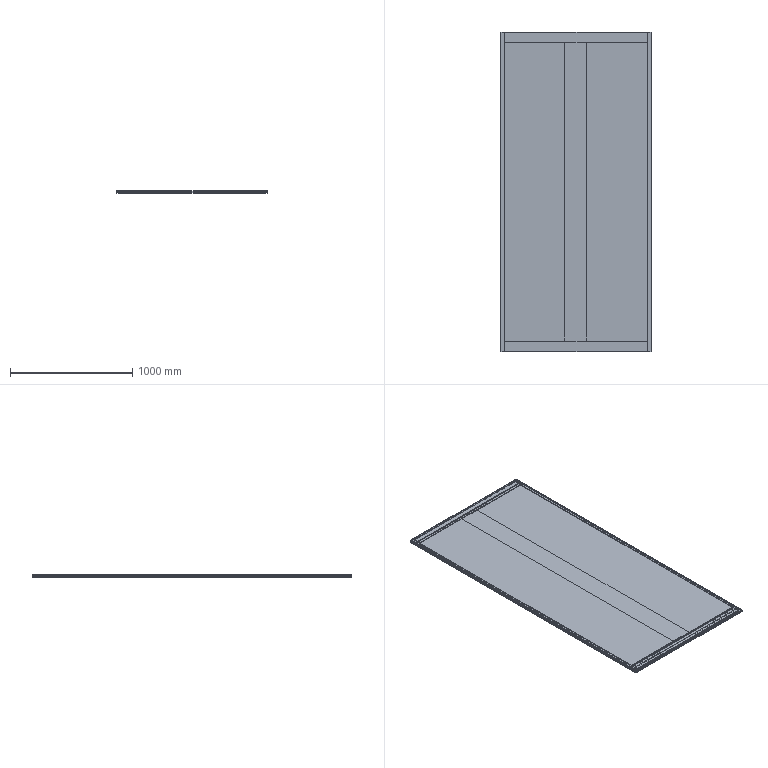Part | 5 solids | 369 faces | box 1230 x 2616 x 20.2 mm | volume 31803633 mm3 | cylinder 187 | plane 182 | commonest cylinder face diameters 0.6 x48 13 x48 0.4 x34 1 x21 9 x16 7.2 x12